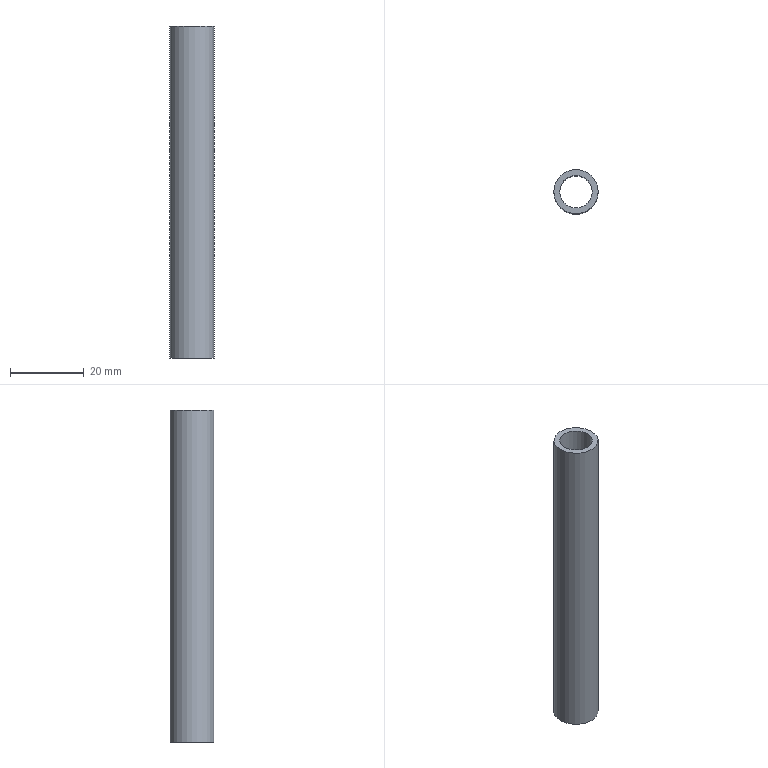Part | STEP file | BS EN ISO 1127(2) - 12 x 1,6 - 100 | 1 solid | 4 faces | box 12 x 12 x 90 mm | volume 4705 mm3 | cylinder 2 | plane 2 | commonest cylinder face diameters 8.8 x1 12 x1
STEP:
#1=CARTESIAN_POINT('',(0.,0.,0.));
#2=DIRECTION('',(0.,0.,1.));
#3=DIRECTION('',(1.,0.,0.));
#4=AXIS2_PLACEMENT_3D('',#1,#2,#3);
#5=CARTESIAN_POINT('',(4.4,0.,90.));
#6=VERTEX_POINT('',#5);
#7=CARTESIAN_POINT('',(0.,0.,90.));
#8=DIRECTION('',(0.,0.,1.));
#9=DIRECTION('',(-1.,0.,0.));
#10=AXIS2_PLACEMENT_3D('',#7,#8,#9);
#11=CIRCLE('',#10,4.4);
#12=CARTESIAN_POINT('',(0.,0.,0.));
#13=DIRECTION('',(0.,0.,1.));
#14=DIRECTION('',(-1.,0.,0.));
#15=AXIS2_PLACEMENT_3D('',#12,#13,#14);
#16=CYLINDRICAL_SURFACE('',#15,4.4);
#17=CARTESIAN_POINT('',(0.,90.));
#18=DIRECTION('',(1.,0.));
#19=VECTOR('',#18,1.);
#20=LINE('',#17,#19);
#21=(GEOMETRIC_REPRESENTATION_CONTEXT(2)PARAMETRIC_REPRESENTATION_CONTEXT()REPRESENTATION_CONTEXT('',''));
#22=DEFINITIONAL_REPRESENTATION('',(#20),#21);
#23=PCURVE('',#16,#22);
#24=CARTESIAN_POINT('',(0.,0.,90.));
#25=DIRECTION('',(0.,0.,1.));
#26=DIRECTION('',(1.,0.,0.));
#27=AXIS2_PLACEMENT_3D('',#24,#25,#26);
#28=PLANE('',#27);
#29=CARTESIAN_POINT('',(0.,0.));
#30=DIRECTION('',(-1.,0.));
#31=AXIS2_PLACEMENT_2D('',#29,#30);
#32=CIRCLE('',#31,4.4);
#33=(GEOMETRIC_REPRESENTATION_CONTEXT(2)PARAMETRIC_REPRESENTATION_CONTEXT()REPRESENTATION_CONTEXT('',''));
#34=DEFINITIONAL_REPRESENTATION('',(#32),#33);
#35=PCURVE('',#28,#34);
#36=SURFACE_CURVE('',#11,(#23,#35),.PCURVE_S1.);
#37=EDGE_CURVE('',#6,#6,#36,.T.);
#38=ORIENTED_EDGE('',*,*,#37,.F.);
#39=CARTESIAN_POINT('',(4.4,0.,0.));
#40=VERTEX_POINT('',#39);
#41=CARTESIAN_POINT('',(4.4,0.,0.));
#42=CARTESIAN_POINT('',(4.4,0.,90.));
#43=B_SPLINE_CURVE_WITH_KNOTS('',1,(#41,#42),.UNSPECIFIED.,.F.,.F.,(2,2),(0.,90.),.PIECEWISE_BEZIER_KNOTS.);
#44=CARTESIAN_POINT('',(3.142,0.));
#45=DIRECTION('',(0.,1.));
#46=VECTOR('',#45,1.);
#47=LINE('',#44,#46);
#48=(GEOMETRIC_REPRESENTATION_CONTEXT(2)PARAMETRIC_REPRESENTATION_CONTEXT()REPRESENTATION_CONTEXT('',''));
#49=DEFINITIONAL_REPRESENTATION('',(#47),#48);
#50=PCURVE('',#16,#49);
#51=CARTESIAN_POINT('',(9.425,0.));
#52=DIRECTION('',(0.,1.));
#53=VECTOR('',#52,1.);
#54=LINE('',#51,#53);
#55=(GEOMETRIC_REPRESENTATION_CONTEXT(2)PARAMETRIC_REPRESENTATION_CONTEXT()REPRESENTATION_CONTEXT('',''));
#56=DEFINITIONAL_REPRESENTATION('',(#54),#55);
#57=PCURVE('',#16,#56);
#58=SEAM_CURVE('',#43,(#50,#57),.PCURVE_S1.);
#59=EDGE_CURVE('',#40,#6,#58,.T.);
#60=ORIENTED_EDGE('',*,*,#59,.F.);
#61=CARTESIAN_POINT('',(0.,0.,0.));
#62=DIRECTION('',(0.,0.,1.));
#63=DIRECTION('',(-1.,0.,0.));
#64=AXIS2_PLACEMENT_3D('',#61,#62,#63);
#65=CIRCLE('',#64,4.4);
#66=CARTESIAN_POINT('',(0.,0.));
#67=DIRECTION('',(1.,0.));
#68=VECTOR('',#67,1.);
#69=LINE('',#66,#68);
#70=(GEOMETRIC_REPRESENTATION_CONTEXT(2)PARAMETRIC_REPRESENTATION_CONTEXT()REPRESENTATION_CONTEXT('',''));
#71=DEFINITIONAL_REPRESENTATION('',(#69),#70);
#72=PCURVE('',#16,#71);
#73=CARTESIAN_POINT('',(0.,0.,0.));
#74=DIRECTION('',(0.,0.,1.));
#75=DIRECTION('',(1.,0.,0.));
#76=AXIS2_PLACEMENT_3D('',#73,#74,#75);
#77=PLANE('',#76);
#78=CARTESIAN_POINT('',(0.,0.));
#79=DIRECTION('',(-1.,0.));
#80=AXIS2_PLACEMENT_2D('',#78,#79);
#81=CIRCLE('',#80,4.4);
#82=(GEOMETRIC_REPRESENTATION_CONTEXT(2)PARAMETRIC_REPRESENTATION_CONTEXT()REPRESENTATION_CONTEXT('',''));
#83=DEFINITIONAL_REPRESENTATION('',(#81),#82);
#84=PCURVE('',#77,#83);
#85=SURFACE_CURVE('',#65,(#72,#84),.PCURVE_S1.);
#86=EDGE_CURVE('',#40,#40,#85,.T.);
#87=ORIENTED_EDGE('',*,*,#86,.T.);
#88=ORIENTED_EDGE('',*,*,#59,.T.);
#89=EDGE_LOOP('',(#38,#60,#87,#88));
#90=FACE_BOUND('',#89,.F.);
#91=ADVANCED_FACE('',(#90),#16,.F.);
#92=CARTESIAN_POINT('',(6.,0.,90.));
#93=VERTEX_POINT('',#92);
#94=CARTESIAN_POINT('',(0.,0.,90.));
#95=DIRECTION('',(0.,0.,-1.));
#96=DIRECTION('',(-1.,0.,0.));
#97=AXIS2_PLACEMENT_3D('',#94,#95,#96);
#98=CIRCLE('',#97,6.);
#99=CARTESIAN_POINT('',(0.,0.,0.));
#100=DIRECTION('',(0.,0.,1.));
#101=DIRECTION('',(-1.,0.,0.));
#102=AXIS2_PLACEMENT_3D('',#99,#100,#101);
#103=CYLINDRICAL_SURFACE('',#102,6.);
#104=CARTESIAN_POINT('',(12.566,90.));
#105=DIRECTION('',(-1.,0.));
#106=VECTOR('',#105,1.);
#107=LINE('',#104,#106);
#108=(GEOMETRIC_REPRESENTATION_CONTEXT(2)PARAMETRIC_REPRESENTATION_CONTEXT()REPRESENTATION_CONTEXT('',''));
#109=DEFINITIONAL_REPRESENTATION('',(#107),#108);
#110=PCURVE('',#103,#109);
#111=CARTESIAN_POINT('',(-6.,0.));
#112=CARTESIAN_POINT('',(-6.,10.392));
#113=CARTESIAN_POINT('',(3.,5.196));
#114=CARTESIAN_POINT('',(12.,0.));
#115=CARTESIAN_POINT('',(3.,-5.196));
#116=CARTESIAN_POINT('',(-6.,-10.392));
#117=CARTESIAN_POINT('',(-6.,0.));
#118=(BOUNDED_CURVE()B_SPLINE_CURVE(2,(#111,#112,#113,#114,#115,#116,#117),.UNSPECIFIED.,.T.,.F.)B_SPLINE_CURVE_WITH_KNOTS((1,2,2,2,2,1),(-2.094,0.,2.094,4.189,6.283,8.378),.UNSPECIFIED.)CURVE()GEOMETRIC_REPRESENTATION_ITEM()RATIONAL_B_SPLINE_CURVE((1.,0.5,1.,0.5,1.,0.5,1.))REPRESENTATION_ITEM(''));
#119=(GEOMETRIC_REPRESENTATION_CONTEXT(2)PARAMETRIC_REPRESENTATION_CONTEXT()REPRESENTATION_CONTEXT('',''));
#120=DEFINITIONAL_REPRESENTATION('',(#118),#119);
#121=PCURVE('',#28,#120);
#122=SURFACE_CURVE('',#98,(#110,#121),.PCURVE_S1.);
#123=EDGE_CURVE('',#93,#93,#122,.T.);
#124=ORIENTED_EDGE('',*,*,#123,.T.);
#125=CARTESIAN_POINT('',(6.,0.,0.));
#126=VERTEX_POINT('',#125);
#127=CARTESIAN_POINT('',(6.,0.,0.));
#128=CARTESIAN_POINT('',(6.,0.,90.));
#129=B_SPLINE_CURVE_WITH_KNOTS('',1,(#127,#128),.UNSPECIFIED.,.F.,.F.,(2,2),(0.,90.),.PIECEWISE_BEZIER_KNOTS.);
#130=CARTESIAN_POINT('',(3.142,0.));
#131=DIRECTION('',(0.,1.));
#132=VECTOR('',#131,1.);
#133=LINE('',#130,#132);
#134=(GEOMETRIC_REPRESENTATION_CONTEXT(2)PARAMETRIC_REPRESENTATION_CONTEXT()REPRESENTATION_CONTEXT('',''));
#135=DEFINITIONAL_REPRESENTATION('',(#133),#134);
#136=PCURVE('',#103,#135);
#137=CARTESIAN_POINT('',(9.425,0.));
#138=DIRECTION('',(0.,1.));
#139=VECTOR('',#138,1.);
#140=LINE('',#137,#139);
#141=(GEOMETRIC_REPRESENTATION_CONTEXT(2)PARAMETRIC_REPRESENTATION_CONTEXT()REPRESENTATION_CONTEXT('',''));
#142=DEFINITIONAL_REPRESENTATION('',(#140),#141);
#143=PCURVE('',#103,#142);
#144=SEAM_CURVE('',#129,(#136,#143),.PCURVE_S1.);
#145=EDGE_CURVE('',#126,#93,#144,.T.);
#146=ORIENTED_EDGE('',*,*,#145,.F.);
#147=CARTESIAN_POINT('',(0.,0.,0.));
#148=DIRECTION('',(0.,0.,-1.));
#149=DIRECTION('',(-1.,0.,0.));
#150=AXIS2_PLACEMENT_3D('',#147,#148,#149);
#151=CIRCLE('',#150,6.);
#152=CARTESIAN_POINT('',(12.566,0.));
#153=DIRECTION('',(-1.,0.));
#154=VECTOR('',#153,1.);
#155=LINE('',#152,#154);
#156=(GEOMETRIC_REPRESENTATION_CONTEXT(2)PARAMETRIC_REPRESENTATION_CONTEXT()REPRESENTATION_CONTEXT('',''));
#157=DEFINITIONAL_REPRESENTATION('',(#155),#156);
#158=PCURVE('',#103,#157);
#159=CARTESIAN_POINT('',(-6.,0.));
#160=CARTESIAN_POINT('',(-6.,10.392));
#161=CARTESIAN_POINT('',(3.,5.196));
#162=CARTESIAN_POINT('',(12.,0.));
#163=CARTESIAN_POINT('',(3.,-5.196));
#164=CARTESIAN_POINT('',(-6.,-10.392));
#165=CARTESIAN_POINT('',(-6.,0.));
#166=(BOUNDED_CURVE()B_SPLINE_CURVE(2,(#159,#160,#161,#162,#163,#164,#165),.UNSPECIFIED.,.T.,.F.)B_SPLINE_CURVE_WITH_KNOTS((1,2,2,2,2,1),(-2.094,0.,2.094,4.189,6.283,8.378),.UNSPECIFIED.)CURVE()GEOMETRIC_REPRESENTATION_ITEM()RATIONAL_B_SPLINE_CURVE((1.,0.5,1.,0.5,1.,0.5,1.))REPRESENTATION_ITEM(''));
#167=(GEOMETRIC_REPRESENTATION_CONTEXT(2)PARAMETRIC_REPRESENTATION_CONTEXT()REPRESENTATION_CONTEXT('',''));
#168=DEFINITIONAL_REPRESENTATION('',(#166),#167);
#169=PCURVE('',#77,#168);
#170=SURFACE_CURVE('',#151,(#158,#169),.PCURVE_S1.);
#171=EDGE_CURVE('',#126,#126,#170,.T.);
#172=ORIENTED_EDGE('',*,*,#171,.F.);
#173=ORIENTED_EDGE('',*,*,#145,.T.);
#174=EDGE_LOOP('',(#124,#146,#172,#173));
#175=FACE_BOUND('',#174,.T.);
#176=ADVANCED_FACE('',(#175),#103,.T.);
#177=ORIENTED_EDGE('',*,*,#171,.T.);
#178=EDGE_LOOP('',(#177));
#179=FACE_BOUND('',#178,.T.);
#180=ORIENTED_EDGE('',*,*,#86,.T.);
#181=EDGE_LOOP('',(#180));
#182=FACE_BOUND('',#181,.T.);
#183=ADVANCED_FACE('',(#179,#182),#77,.F.);
#184=ORIENTED_EDGE('',*,*,#123,.F.);
#185=EDGE_LOOP('',(#184));
#186=FACE_BOUND('',#185,.T.);
#187=ORIENTED_EDGE('',*,*,#37,.F.);
#188=EDGE_LOOP('',(#187));
#189=FACE_BOUND('',#188,.T.);
#190=ADVANCED_FACE('',(#186,#189),#28,.T.);
#191=CLOSED_SHELL('',(#91,#176,#183,#190));
#192=MANIFOLD_SOLID_BREP('',#191);
#193=(LENGTH_UNIT()NAMED_UNIT(*)SI_UNIT(.MILLI.,.METRE.));
#194=UNCERTAINTY_MEASURE_WITH_UNIT(LENGTH_MEASURE(0.00001),#193,'','');
#195=(NAMED_UNIT(*)PLANE_ANGLE_UNIT()SI_UNIT($,.RADIAN.));
#196=(NAMED_UNIT(*)SI_UNIT($,.STERADIAN.)SOLID_ANGLE_UNIT());
#197=(GEOMETRIC_REPRESENTATION_CONTEXT(3)GLOBAL_UNCERTAINTY_ASSIGNED_CONTEXT((#194))GLOBAL_UNIT_ASSIGNED_CONTEXT((#193,#195,#196))REPRESENTATION_CONTEXT('',''));
#198=ADVANCED_BREP_SHAPE_REPRESENTATION('',(#4,#192),#197);